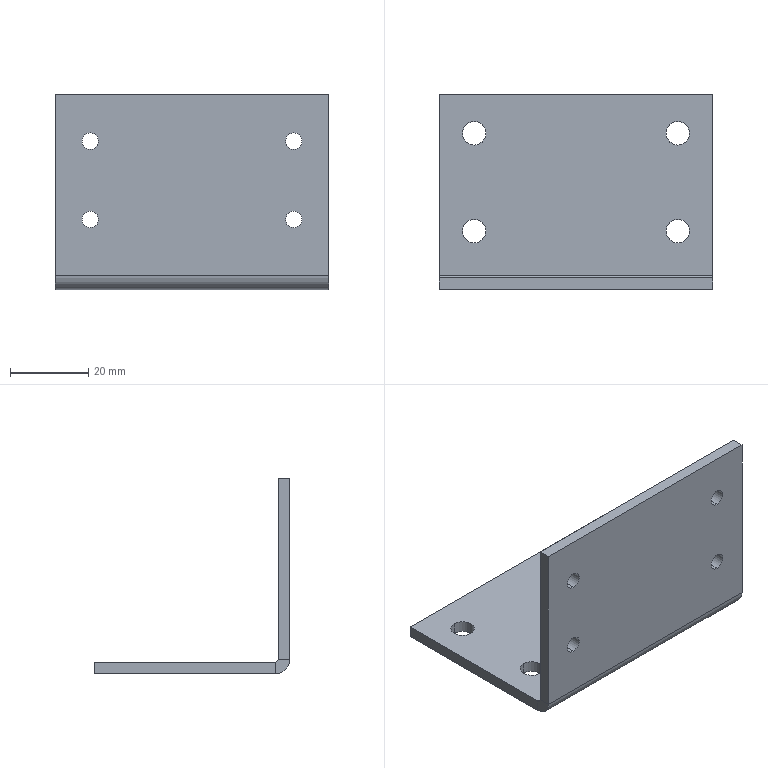Part | STEP file | 3050 drag chain bracket | 1 solid | 30 faces | box 70 x 50 x 50 mm | volume 19663 mm3 | cylinder 18 | plane 12 | commonest cylinder face diameters 4.2 x8 6 x8 1.473 x1 7.473 x1